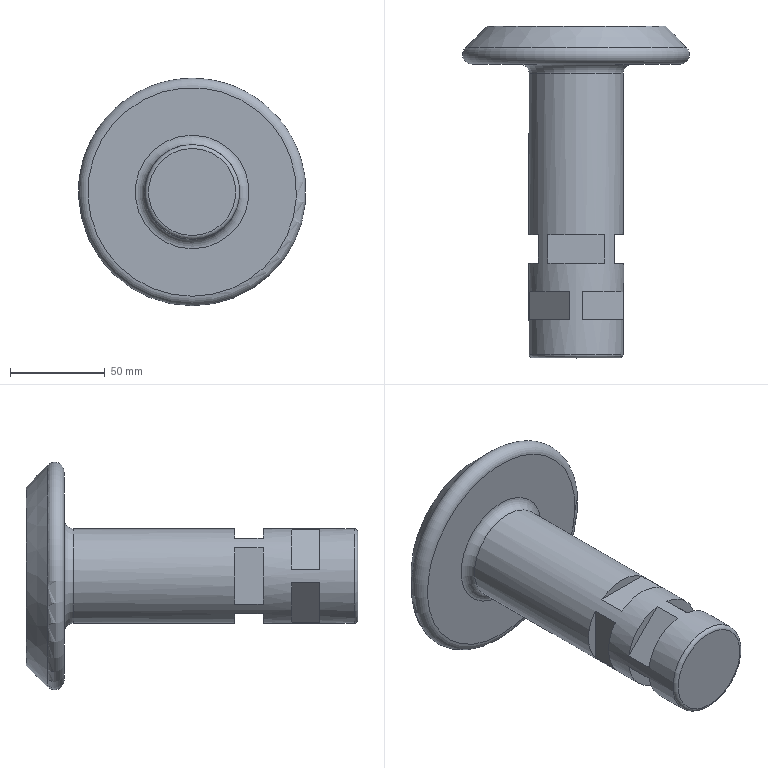Part | NX | features solid 2 | 1 solid | 32 faces | box 120 x 175 x 120 mm | volume 487590 mm3 | plane 27 | torus 3 | cylinder 1 | cone 1 | commonest cylinder face diameters 50 x1
STEP:
#1=CARTESIAN_POINT('',(745.,430.,-50.));
#2=VERTEX_POINT('',#1);
#3=CARTESIAN_POINT('',(745.,430.,-75.));
#4=DIRECTION('',(0.,-1.,0.));
#5=DIRECTION('',(0.,0.,1.));
#6=AXIS2_PLACEMENT_3D('',#3,#4,#5);
#7=CIRCLE('',#6,25.);
#8=EDGE_CURVE('',#2,#2,#7,.F.);
#9=ORIENTED_EDGE('',*,*,#8,.F.);
#10=EDGE_LOOP('',(#9));
#11=FACE_BOUND('',#10,.T.);
#12=CARTESIAN_POINT('',(741.464,300.,-50.251));
#13=VERTEX_POINT('',#12);
#14=CARTESIAN_POINT('',(741.464,315.,-50.251));
#15=VERTEX_POINT('',#14);
#16=CARTESIAN_POINT('',(741.464,435.,-50.251));
#17=DIRECTION('',(0.,-1.,0.));
#18=VECTOR('',#17,1000.);
#19=LINE('',#16,#18);
#20=EDGE_CURVE('',#13,#15,#19,.F.);
#21=ORIENTED_EDGE('',*,*,#20,.F.);
#22=CARTESIAN_POINT('',(720.251,300.,-71.464));
#23=VERTEX_POINT('',#22);
#24=CARTESIAN_POINT('',(745.,300.,-75.));
#25=DIRECTION('',(0.,-1.,0.));
#26=DIRECTION('',(0.,0.,1.));
#27=AXIS2_PLACEMENT_3D('',#24,#25,#26);
#28=CIRCLE('',#27,25.);
#29=EDGE_CURVE('',#23,#13,#28,.F.);
#30=ORIENTED_EDGE('',*,*,#29,.F.);
#31=CARTESIAN_POINT('',(720.251,315.,-71.464));
#32=VERTEX_POINT('',#31);
#33=CARTESIAN_POINT('',(720.251,435.,-71.464));
#34=DIRECTION('',(0.,-1.,0.));
#35=VECTOR('',#34,1000.);
#36=LINE('',#33,#35);
#37=EDGE_CURVE('',#32,#23,#36,.T.);
#38=ORIENTED_EDGE('',*,*,#37,.F.);
#39=CARTESIAN_POINT('',(745.,315.,-75.));
#40=DIRECTION('',(0.,-1.,0.));
#41=DIRECTION('',(0.,0.,1.));
#42=AXIS2_PLACEMENT_3D('',#39,#40,#41);
#43=CIRCLE('',#42,25.);
#44=EDGE_CURVE('',#15,#32,#43,.T.);
#45=ORIENTED_EDGE('',*,*,#44,.F.);
#46=EDGE_LOOP('',(#21,#30,#38,#45));
#47=FACE_BOUND('',#46,.T.);
#48=CARTESIAN_POINT('',(720.251,300.,-78.536));
#49=VERTEX_POINT('',#48);
#50=CARTESIAN_POINT('',(720.251,315.,-78.536));
#51=VERTEX_POINT('',#50);
#52=CARTESIAN_POINT('',(720.251,435.,-78.536));
#53=DIRECTION('',(0.,-1.,0.));
#54=VECTOR('',#53,1000.);
#55=LINE('',#52,#54);
#56=EDGE_CURVE('',#49,#51,#55,.F.);
#57=ORIENTED_EDGE('',*,*,#56,.F.);
#58=CARTESIAN_POINT('',(741.464,300.,-99.749));
#59=VERTEX_POINT('',#58);
#60=CARTESIAN_POINT('',(745.,300.,-75.));
#61=DIRECTION('',(0.,-1.,0.));
#62=DIRECTION('',(0.,0.,1.));
#63=AXIS2_PLACEMENT_3D('',#60,#61,#62);
#64=CIRCLE('',#63,25.);
#65=EDGE_CURVE('',#59,#49,#64,.F.);
#66=ORIENTED_EDGE('',*,*,#65,.F.);
#67=CARTESIAN_POINT('',(741.464,315.,-99.749));
#68=VERTEX_POINT('',#67);
#69=CARTESIAN_POINT('',(741.464,435.,-99.749));
#70=DIRECTION('',(0.,-1.,0.));
#71=VECTOR('',#70,1000.);
#72=LINE('',#69,#71);
#73=EDGE_CURVE('',#68,#59,#72,.T.);
#74=ORIENTED_EDGE('',*,*,#73,.F.);
#75=CARTESIAN_POINT('',(745.,315.,-75.));
#76=DIRECTION('',(0.,-1.,0.));
#77=DIRECTION('',(0.,0.,1.));
#78=AXIS2_PLACEMENT_3D('',#75,#76,#77);
#79=CIRCLE('',#78,25.);
#80=EDGE_CURVE('',#51,#68,#79,.T.);
#81=ORIENTED_EDGE('',*,*,#80,.F.);
#82=EDGE_LOOP('',(#57,#66,#74,#81));
#83=FACE_BOUND('',#82,.T.);
#84=CARTESIAN_POINT('',(725.,330.,-60.));
#85=VERTEX_POINT('',#84);
#86=CARTESIAN_POINT('',(725.,345.,-60.));
#87=VERTEX_POINT('',#86);
#88=CARTESIAN_POINT('',(725.,435.,-60.));
#89=DIRECTION('',(0.,-1.,0.));
#90=VECTOR('',#89,1000.);
#91=LINE('',#88,#90);
#92=EDGE_CURVE('',#85,#87,#91,.F.);
#93=ORIENTED_EDGE('',*,*,#92,.F.);
#94=CARTESIAN_POINT('',(725.,330.,-90.));
#95=VERTEX_POINT('',#94);
#96=CARTESIAN_POINT('',(745.,330.,-75.));
#97=DIRECTION('',(0.,-1.,0.));
#98=DIRECTION('',(0.,0.,1.));
#99=AXIS2_PLACEMENT_3D('',#96,#97,#98);
#100=CIRCLE('',#99,25.);
#101=EDGE_CURVE('',#95,#85,#100,.F.);
#102=ORIENTED_EDGE('',*,*,#101,.F.);
#103=CARTESIAN_POINT('',(725.,345.,-90.));
#104=VERTEX_POINT('',#103);
#105=CARTESIAN_POINT('',(725.,435.,-90.));
#106=DIRECTION('',(0.,-1.,0.));
#107=VECTOR('',#106,1000.);
#108=LINE('',#105,#107);
#109=EDGE_CURVE('',#104,#95,#108,.T.);
#110=ORIENTED_EDGE('',*,*,#109,.F.);
#111=CARTESIAN_POINT('',(745.,345.,-75.));
#112=DIRECTION('',(0.,-1.,0.));
#113=DIRECTION('',(0.,0.,1.));
#114=AXIS2_PLACEMENT_3D('',#111,#112,#113);
#115=CIRCLE('',#114,25.);
#116=EDGE_CURVE('',#87,#104,#115,.T.);
#117=ORIENTED_EDGE('',*,*,#116,.F.);
#118=EDGE_LOOP('',(#93,#102,#110,#117));
#119=FACE_BOUND('',#118,.T.);
#120=CARTESIAN_POINT('',(760.,345.,-55.));
#121=VERTEX_POINT('',#120);
#122=CARTESIAN_POINT('',(730.,345.,-55.));
#123=VERTEX_POINT('',#122);
#124=CARTESIAN_POINT('',(745.,345.,-75.));
#125=DIRECTION('',(0.,-1.,0.));
#126=DIRECTION('',(0.,0.,1.));
#127=AXIS2_PLACEMENT_3D('',#124,#125,#126);
#128=CIRCLE('',#127,25.);
#129=EDGE_CURVE('',#121,#123,#128,.T.);
#130=ORIENTED_EDGE('',*,*,#129,.F.);
#131=CARTESIAN_POINT('',(760.,330.,-55.));
#132=VERTEX_POINT('',#131);
#133=CARTESIAN_POINT('',(760.,435.,-55.));
#134=DIRECTION('',(0.,-1.,0.));
#135=VECTOR('',#134,1000.);
#136=LINE('',#133,#135);
#137=EDGE_CURVE('',#132,#121,#136,.F.);
#138=ORIENTED_EDGE('',*,*,#137,.F.);
#139=CARTESIAN_POINT('',(730.,330.,-55.));
#140=VERTEX_POINT('',#139);
#141=CARTESIAN_POINT('',(745.,330.,-75.));
#142=DIRECTION('',(0.,-1.,0.));
#143=DIRECTION('',(0.,0.,1.));
#144=AXIS2_PLACEMENT_3D('',#141,#142,#143);
#145=CIRCLE('',#144,25.);
#146=EDGE_CURVE('',#140,#132,#145,.F.);
#147=ORIENTED_EDGE('',*,*,#146,.F.);
#148=CARTESIAN_POINT('',(730.,435.,-55.));
#149=DIRECTION('',(0.,-1.,0.));
#150=VECTOR('',#149,1000.);
#151=LINE('',#148,#150);
#152=EDGE_CURVE('',#123,#140,#151,.T.);
#153=ORIENTED_EDGE('',*,*,#152,.F.);
#154=EDGE_LOOP('',(#130,#138,#147,#153));
#155=FACE_BOUND('',#154,.T.);
#156=CARTESIAN_POINT('',(745.,282.,-50.));
#157=VERTEX_POINT('',#156);
#158=CARTESIAN_POINT('',(745.,282.,-75.));
#159=DIRECTION('',(0.,-1.,0.));
#160=DIRECTION('',(0.,0.,1.));
#161=AXIS2_PLACEMENT_3D('',#158,#159,#160);
#162=CIRCLE('',#161,25.);
#163=EDGE_CURVE('',#157,#157,#162,.T.);
#164=ORIENTED_EDGE('',*,*,#163,.F.);
#165=EDGE_LOOP('',(#164));
#166=FACE_BOUND('',#165,.T.);
#167=CARTESIAN_POINT('',(760.,345.,-95.));
#168=VERTEX_POINT('',#167);
#169=CARTESIAN_POINT('',(730.,345.,-95.));
#170=VERTEX_POINT('',#169);
#171=CARTESIAN_POINT('',(745.,345.,-75.));
#172=DIRECTION('',(0.,-1.,0.));
#173=DIRECTION('',(0.,0.,1.));
#174=AXIS2_PLACEMENT_3D('',#171,#172,#173);
#175=CIRCLE('',#174,25.);
#176=EDGE_CURVE('',#168,#170,#175,.F.);
#177=ORIENTED_EDGE('',*,*,#176,.T.);
#178=CARTESIAN_POINT('',(730.,330.,-95.));
#179=VERTEX_POINT('',#178);
#180=CARTESIAN_POINT('',(730.,435.,-95.));
#181=DIRECTION('',(0.,-1.,0.));
#182=VECTOR('',#181,1000.);
#183=LINE('',#180,#182);
#184=EDGE_CURVE('',#170,#179,#183,.T.);
#185=ORIENTED_EDGE('',*,*,#184,.T.);
#186=CARTESIAN_POINT('',(760.,330.,-95.));
#187=VERTEX_POINT('',#186);
#188=CARTESIAN_POINT('',(745.,330.,-75.));
#189=DIRECTION('',(0.,-1.,0.));
#190=DIRECTION('',(0.,0.,1.));
#191=AXIS2_PLACEMENT_3D('',#188,#189,#190);
#192=CIRCLE('',#191,25.);
#193=EDGE_CURVE('',#179,#187,#192,.T.);
#194=ORIENTED_EDGE('',*,*,#193,.T.);
#195=CARTESIAN_POINT('',(760.,435.,-95.));
#196=DIRECTION('',(0.,-1.,0.));
#197=VECTOR('',#196,1000.);
#198=LINE('',#195,#197);
#199=EDGE_CURVE('',#187,#168,#198,.F.);
#200=ORIENTED_EDGE('',*,*,#199,.T.);
#201=EDGE_LOOP('',(#177,#185,#194,#200));
#202=FACE_BOUND('',#201,.T.);
#203=CARTESIAN_POINT('',(765.,345.,-60.));
#204=VERTEX_POINT('',#203);
#205=CARTESIAN_POINT('',(765.,345.,-90.));
#206=VERTEX_POINT('',#205);
#207=CARTESIAN_POINT('',(745.,345.,-75.));
#208=DIRECTION('',(0.,-1.,0.));
#209=DIRECTION('',(0.,0.,1.));
#210=AXIS2_PLACEMENT_3D('',#207,#208,#209);
#211=CIRCLE('',#210,25.);
#212=EDGE_CURVE('',#204,#206,#211,.F.);
#213=ORIENTED_EDGE('',*,*,#212,.T.);
#214=CARTESIAN_POINT('',(765.,330.,-90.));
#215=VERTEX_POINT('',#214);
#216=CARTESIAN_POINT('',(765.,435.,-90.));
#217=DIRECTION('',(0.,-1.,0.));
#218=VECTOR('',#217,1000.);
#219=LINE('',#216,#218);
#220=EDGE_CURVE('',#206,#215,#219,.T.);
#221=ORIENTED_EDGE('',*,*,#220,.T.);
#222=CARTESIAN_POINT('',(765.,330.,-60.));
#223=VERTEX_POINT('',#222);
#224=CARTESIAN_POINT('',(745.,330.,-75.));
#225=DIRECTION('',(0.,-1.,0.));
#226=DIRECTION('',(0.,0.,1.));
#227=AXIS2_PLACEMENT_3D('',#224,#225,#226);
#228=CIRCLE('',#227,25.);
#229=EDGE_CURVE('',#215,#223,#228,.T.);
#230=ORIENTED_EDGE('',*,*,#229,.T.);
#231=CARTESIAN_POINT('',(765.,435.,-60.));
#232=DIRECTION('',(0.,-1.,0.));
#233=VECTOR('',#232,1000.);
#234=LINE('',#231,#233);
#235=EDGE_CURVE('',#223,#204,#234,.F.);
#236=ORIENTED_EDGE('',*,*,#235,.T.);
#237=EDGE_LOOP('',(#213,#221,#230,#236));
#238=FACE_BOUND('',#237,.T.);
#239=CARTESIAN_POINT('',(748.536,315.,-50.251));
#240=VERTEX_POINT('',#239);
#241=CARTESIAN_POINT('',(769.749,315.,-71.464));
#242=VERTEX_POINT('',#241);
#243=CARTESIAN_POINT('',(745.,315.,-75.));
#244=DIRECTION('',(0.,-1.,0.));
#245=DIRECTION('',(0.,0.,1.));
#246=AXIS2_PLACEMENT_3D('',#243,#244,#245);
#247=CIRCLE('',#246,25.);
#248=EDGE_CURVE('',#240,#242,#247,.F.);
#249=ORIENTED_EDGE('',*,*,#248,.T.);
#250=CARTESIAN_POINT('',(769.749,300.,-71.464));
#251=VERTEX_POINT('',#250);
#252=CARTESIAN_POINT('',(769.749,435.,-71.464));
#253=DIRECTION('',(0.,-1.,0.));
#254=VECTOR('',#253,1000.);
#255=LINE('',#252,#254);
#256=EDGE_CURVE('',#242,#251,#255,.T.);
#257=ORIENTED_EDGE('',*,*,#256,.T.);
#258=CARTESIAN_POINT('',(748.536,300.,-50.251));
#259=VERTEX_POINT('',#258);
#260=CARTESIAN_POINT('',(745.,300.,-75.));
#261=DIRECTION('',(0.,-1.,0.));
#262=DIRECTION('',(0.,0.,1.));
#263=AXIS2_PLACEMENT_3D('',#260,#261,#262);
#264=CIRCLE('',#263,25.);
#265=EDGE_CURVE('',#251,#259,#264,.T.);
#266=ORIENTED_EDGE('',*,*,#265,.T.);
#267=CARTESIAN_POINT('',(748.536,435.,-50.251));
#268=DIRECTION('',(0.,-1.,0.));
#269=VECTOR('',#268,1000.);
#270=LINE('',#267,#269);
#271=EDGE_CURVE('',#259,#240,#270,.F.);
#272=ORIENTED_EDGE('',*,*,#271,.T.);
#273=EDGE_LOOP('',(#249,#257,#266,#272));
#274=FACE_BOUND('',#273,.T.);
#275=CARTESIAN_POINT('',(769.749,315.,-78.536));
#276=VERTEX_POINT('',#275);
#277=CARTESIAN_POINT('',(748.536,315.,-99.749));
#278=VERTEX_POINT('',#277);
#279=CARTESIAN_POINT('',(745.,315.,-75.));
#280=DIRECTION('',(0.,-1.,0.));
#281=DIRECTION('',(0.,0.,1.));
#282=AXIS2_PLACEMENT_3D('',#279,#280,#281);
#283=CIRCLE('',#282,25.);
#284=EDGE_CURVE('',#276,#278,#283,.F.);
#285=ORIENTED_EDGE('',*,*,#284,.T.);
#286=CARTESIAN_POINT('',(748.536,300.,-99.749));
#287=VERTEX_POINT('',#286);
#288=CARTESIAN_POINT('',(748.536,435.,-99.749));
#289=DIRECTION('',(0.,-1.,0.));
#290=VECTOR('',#289,1000.);
#291=LINE('',#288,#290);
#292=EDGE_CURVE('',#278,#287,#291,.T.);
#293=ORIENTED_EDGE('',*,*,#292,.T.);
#294=CARTESIAN_POINT('',(769.749,300.,-78.536));
#295=VERTEX_POINT('',#294);
#296=CARTESIAN_POINT('',(745.,300.,-75.));
#297=DIRECTION('',(0.,-1.,0.));
#298=DIRECTION('',(0.,0.,1.));
#299=AXIS2_PLACEMENT_3D('',#296,#297,#298);
#300=CIRCLE('',#299,25.);
#301=EDGE_CURVE('',#287,#295,#300,.T.);
#302=ORIENTED_EDGE('',*,*,#301,.T.);
#303=CARTESIAN_POINT('',(769.749,435.,-78.536));
#304=DIRECTION('',(0.,-1.,0.));
#305=VECTOR('',#304,1000.);
#306=LINE('',#303,#305);
#307=EDGE_CURVE('',#295,#276,#306,.F.);
#308=ORIENTED_EDGE('',*,*,#307,.T.);
#309=EDGE_LOOP('',(#285,#293,#302,#308));
#310=FACE_BOUND('',#309,.T.);
#311=CARTESIAN_POINT('',(745.,435.,-75.));
#312=DIRECTION('',(0.,-1.,0.));
#313=DIRECTION('',(0.,0.,-1.));
#314=AXIS2_PLACEMENT_3D('',#311,#312,#313);
#315=CYLINDRICAL_SURFACE('',#314,25.);
#316=ADVANCED_FACE('',(#11,#47,#83,#119,#155,#166,#202,#238,#274,#310),#315,.T.);
#317=CARTESIAN_POINT('',(745.,280.,-52.));
#318=VERTEX_POINT('',#317);
#319=CARTESIAN_POINT('',(745.,280.,-75.));
#320=DIRECTION('',(0.,-1.,0.));
#321=DIRECTION('',(0.,0.,1.));
#322=AXIS2_PLACEMENT_3D('',#319,#320,#321);
#323=CIRCLE('',#322,23.);
#324=EDGE_CURVE('',#318,#318,#323,.F.);
#325=ORIENTED_EDGE('',*,*,#324,.F.);
#326=EDGE_LOOP('',(#325));
#327=FACE_BOUND('',#326,.T.);
#328=CARTESIAN_POINT('',(720.,280.,-75.));
#329=DIRECTION('',(0.,1.,0.));
#330=DIRECTION('',(0.,0.,1.));
#331=AXIS2_PLACEMENT_3D('',#328,#329,#330);
#332=PLANE('',#331);
#333=ADVANCED_FACE('',(#327),#332,.F.);
#334=CARTESIAN_POINT('',(745.,435.,-45.));
#335=VERTEX_POINT('',#334);
#336=CARTESIAN_POINT('',(745.,435.,-75.));
#337=DIRECTION('',(0.,-1.,0.));
#338=DIRECTION('',(0.,0.,1.));
#339=AXIS2_PLACEMENT_3D('',#336,#337,#338);
#340=CIRCLE('',#339,30.);
#341=EDGE_CURVE('',#335,#335,#340,.T.);
#342=ORIENTED_EDGE('',*,*,#341,.F.);
#343=EDGE_LOOP('',(#342));
#344=FACE_BOUND('',#343,.T.);
#345=CARTESIAN_POINT('',(745.,435.,-130.));
#346=VERTEX_POINT('',#345);
#347=CARTESIAN_POINT('',(745.,435.,-75.));
#348=DIRECTION('',(0.,1.,0.));
#349=DIRECTION('',(0.,0.,-1.));
#350=AXIS2_PLACEMENT_3D('',#347,#348,#349);
#351=CIRCLE('',#350,55.);
#352=EDGE_CURVE('',#346,#346,#351,.T.);
#353=ORIENTED_EDGE('',*,*,#352,.F.);
#354=EDGE_LOOP('',(#353));
#355=FACE_BOUND('',#354,.T.);
#356=CARTESIAN_POINT('',(690.,435.,-75.));
#357=DIRECTION('',(0.,1.,0.));
#358=DIRECTION('',(0.,0.,1.));
#359=AXIS2_PLACEMENT_3D('',#356,#357,#358);
#360=PLANE('',#359);
#361=ADVANCED_FACE('',(#344,#355),#360,.F.);
#362=CARTESIAN_POINT('',(745.,443.536,-133.536));
#363=VERTEX_POINT('',#362);
#364=CARTESIAN_POINT('',(745.,443.536,-75.));
#365=DIRECTION('',(0.,1.,0.));
#366=DIRECTION('',(0.,0.,-1.));
#367=AXIS2_PLACEMENT_3D('',#364,#365,#366);
#368=CIRCLE('',#367,58.536);
#369=EDGE_CURVE('',#363,#363,#368,.T.);
#370=ORIENTED_EDGE('',*,*,#369,.T.);
#371=EDGE_LOOP('',(#370));
#372=FACE_BOUND('',#371,.T.);
#373=CARTESIAN_POINT('',(745.,455.,-122.071));
#374=VERTEX_POINT('',#373);
#375=CARTESIAN_POINT('',(745.,455.,-75.));
#376=DIRECTION('',(0.,1.,0.));
#377=DIRECTION('',(0.,0.,-1.));
#378=AXIS2_PLACEMENT_3D('',#375,#376,#377);
#379=CIRCLE('',#378,47.071);
#380=EDGE_CURVE('',#374,#374,#379,.T.);
#381=ORIENTED_EDGE('',*,*,#380,.F.);
#382=EDGE_LOOP('',(#381));
#383=FACE_BOUND('',#382,.T.);
#384=CARTESIAN_POINT('',(745.,455.,-75.));
#385=DIRECTION('',(0.,-1.,0.));
#386=DIRECTION('',(0.,0.,-1.));
#387=AXIS2_PLACEMENT_3D('',#384,#385,#386);
#388=CONICAL_SURFACE('',#387,47.071,0.7854);
#389=ADVANCED_FACE('',(#372,#383),#388,.T.);
#390=ORIENTED_EDGE('',*,*,#380,.T.);
#391=EDGE_LOOP('',(#390));
#392=FACE_BOUND('',#391,.T.);
#393=CARTESIAN_POINT('',(745.,455.,-75.));
#394=DIRECTION('',(0.,-1.,0.));
#395=DIRECTION('',(0.,0.,-1.));
#396=AXIS2_PLACEMENT_3D('',#393,#394,#395);
#397=PLANE('',#396);
#398=ADVANCED_FACE('',(#392),#397,.F.);
#399=ORIENTED_EDGE('',*,*,#369,.F.);
#400=EDGE_LOOP('',(#399));
#401=FACE_BOUND('',#400,.T.);
#402=ORIENTED_EDGE('',*,*,#352,.T.);
#403=EDGE_LOOP('',(#402));
#404=FACE_BOUND('',#403,.T.);
#405=CARTESIAN_POINT('',(745.,440.,-75.));
#406=DIRECTION('',(0.,-1.,0.));
#407=DIRECTION('',(0.,0.,-1.));
#408=AXIS2_PLACEMENT_3D('',#405,#406,#407);
#409=TOROIDAL_SURFACE('',#408,55.,5.);
#410=ADVANCED_FACE('',(#401,#404),#409,.T.);
#411=ORIENTED_EDGE('',*,*,#163,.T.);
#412=EDGE_LOOP('',(#411));
#413=FACE_BOUND('',#412,.T.);
#414=ORIENTED_EDGE('',*,*,#324,.T.);
#415=EDGE_LOOP('',(#414));
#416=FACE_BOUND('',#415,.T.);
#417=CARTESIAN_POINT('',(745.,282.,-75.));
#418=DIRECTION('',(0.,1.,0.));
#419=DIRECTION('',(0.,0.,1.));
#420=AXIS2_PLACEMENT_3D('',#417,#418,#419);
#421=TOROIDAL_SURFACE('',#420,23.,2.);
#422=ADVANCED_FACE('',(#413,#416),#421,.T.);
#423=CARTESIAN_POINT('',(765.,345.,-95.));
#424=DIRECTION('',(-1.,0.,0.));
#425=VECTOR('',#424,1000.);
#426=LINE('',#423,#425);
#427=EDGE_CURVE('',#168,#170,#426,.T.);
#428=ORIENTED_EDGE('',*,*,#427,.T.);
#429=ORIENTED_EDGE('',*,*,#176,.F.);
#430=EDGE_LOOP('',(#428,#429));
#431=FACE_BOUND('',#430,.T.);
#432=CARTESIAN_POINT('',(765.,345.,-75.));
#433=DIRECTION('',(0.,1.,0.));
#434=DIRECTION('',(-1.,0.,0.));
#435=AXIS2_PLACEMENT_3D('',#432,#433,#434);
#436=PLANE('',#435);
#437=ADVANCED_FACE('',(#431),#436,.F.);
#438=CARTESIAN_POINT('',(765.,330.,-95.));
#439=DIRECTION('',(-1.,0.,0.));
#440=VECTOR('',#439,1000.);
#441=LINE('',#438,#440);
#442=EDGE_CURVE('',#187,#179,#441,.T.);
#443=ORIENTED_EDGE('',*,*,#442,.F.);
#444=ORIENTED_EDGE('',*,*,#193,.F.);
#445=EDGE_LOOP('',(#443,#444));
#446=FACE_BOUND('',#445,.T.);
#447=CARTESIAN_POINT('',(765.,330.,-75.));
#448=DIRECTION('',(0.,1.,0.));
#449=DIRECTION('',(-1.,0.,0.));
#450=AXIS2_PLACEMENT_3D('',#447,#448,#449);
#451=PLANE('',#450);
#452=ADVANCED_FACE('',(#446),#451,.T.);
#453=ORIENTED_EDGE('',*,*,#184,.F.);
#454=ORIENTED_EDGE('',*,*,#427,.F.);
#455=ORIENTED_EDGE('',*,*,#199,.F.);
#456=ORIENTED_EDGE('',*,*,#442,.T.);
#457=EDGE_LOOP('',(#453,#454,#455,#456));
#458=FACE_BOUND('',#457,.T.);
#459=CARTESIAN_POINT('',(765.,345.,-95.));
#460=DIRECTION('',(0.,0.,-1.));
#461=DIRECTION('',(-1.,0.,0.));
#462=AXIS2_PLACEMENT_3D('',#459,#460,#461);
#463=PLANE('',#462);
#464=ADVANCED_FACE('',(#458),#463,.T.);
#465=ORIENTED_EDGE('',*,*,#129,.T.);
#466=CARTESIAN_POINT('',(765.,345.,-55.));
#467=DIRECTION('',(-1.,0.,0.));
#468=VECTOR('',#467,1000.);
#469=LINE('',#466,#468);
#470=EDGE_CURVE('',#121,#123,#469,.T.);
#471=ORIENTED_EDGE('',*,*,#470,.F.);
#472=EDGE_LOOP('',(#465,#471));
#473=FACE_BOUND('',#472,.T.);
#474=CARTESIAN_POINT('',(765.,345.,-75.));
#475=DIRECTION('',(0.,1.,0.));
#476=DIRECTION('',(-1.,0.,0.));
#477=AXIS2_PLACEMENT_3D('',#474,#475,#476);
#478=PLANE('',#477);
#479=ADVANCED_FACE('',(#473),#478,.F.);
#480=ORIENTED_EDGE('',*,*,#146,.T.);
#481=CARTESIAN_POINT('',(765.,330.,-55.));
#482=DIRECTION('',(-1.,0.,0.));
#483=VECTOR('',#482,1000.);
#484=LINE('',#481,#483);
#485=EDGE_CURVE('',#132,#140,#484,.T.);
#486=ORIENTED_EDGE('',*,*,#485,.T.);
#487=EDGE_LOOP('',(#480,#486));
#488=FACE_BOUND('',#487,.T.);
#489=CARTESIAN_POINT('',(765.,330.,-75.));
#490=DIRECTION('',(0.,1.,0.));
#491=DIRECTION('',(-1.,0.,0.));
#492=AXIS2_PLACEMENT_3D('',#489,#490,#491);
#493=PLANE('',#492);
#494=ADVANCED_FACE('',(#488),#493,.T.);
#495=ORIENTED_EDGE('',*,*,#470,.T.);
#496=ORIENTED_EDGE('',*,*,#152,.T.);
#497=ORIENTED_EDGE('',*,*,#485,.F.);
#498=ORIENTED_EDGE('',*,*,#137,.T.);
#499=EDGE_LOOP('',(#495,#496,#497,#498));
#500=FACE_BOUND('',#499,.T.);
#501=CARTESIAN_POINT('',(765.,345.,-55.));
#502=DIRECTION('',(0.,0.,-1.));
#503=DIRECTION('',(-1.,0.,0.));
#504=AXIS2_PLACEMENT_3D('',#501,#502,#503);
#505=PLANE('',#504);
#506=ADVANCED_FACE('',(#500),#505,.F.);
#507=CARTESIAN_POINT('',(765.,345.,-55.));
#508=DIRECTION('',(0.,0.,-1.));
#509=VECTOR('',#508,1000.);
#510=LINE('',#507,#509);
#511=EDGE_CURVE('',#204,#206,#510,.T.);
#512=ORIENTED_EDGE('',*,*,#511,.T.);
#513=ORIENTED_EDGE('',*,*,#212,.F.);
#514=EDGE_LOOP('',(#512,#513));
#515=FACE_BOUND('',#514,.T.);
#516=CARTESIAN_POINT('',(745.,345.,-55.));
#517=DIRECTION('',(0.,1.,0.));
#518=DIRECTION('',(0.,0.,-1.));
#519=AXIS2_PLACEMENT_3D('',#516,#517,#518);
#520=PLANE('',#519);
#521=ADVANCED_FACE('',(#515),#520,.F.);
#522=CARTESIAN_POINT('',(765.,330.,-55.));
#523=DIRECTION('',(0.,0.,-1.));
#524=VECTOR('',#523,1000.);
#525=LINE('',#522,#524);
#526=EDGE_CURVE('',#223,#215,#525,.T.);
#527=ORIENTED_EDGE('',*,*,#526,.F.);
#528=ORIENTED_EDGE('',*,*,#229,.F.);
#529=EDGE_LOOP('',(#527,#528));
#530=FACE_BOUND('',#529,.T.);
#531=CARTESIAN_POINT('',(745.,330.,-55.));
#532=DIRECTION('',(0.,1.,0.));
#533=DIRECTION('',(0.,0.,-1.));
#534=AXIS2_PLACEMENT_3D('',#531,#532,#533);
#535=PLANE('',#534);
#536=ADVANCED_FACE('',(#530),#535,.T.);
#537=ORIENTED_EDGE('',*,*,#220,.F.);
#538=ORIENTED_EDGE('',*,*,#511,.F.);
#539=ORIENTED_EDGE('',*,*,#235,.F.);
#540=ORIENTED_EDGE('',*,*,#526,.T.);
#541=EDGE_LOOP('',(#537,#538,#539,#540));
#542=FACE_BOUND('',#541,.T.);
#543=CARTESIAN_POINT('',(765.,345.,-55.));
#544=DIRECTION('',(1.,0.,0.));
#545=DIRECTION('',(0.,0.,-1.));
#546=AXIS2_PLACEMENT_3D('',#543,#544,#545);
#547=PLANE('',#546);
#548=ADVANCED_FACE('',(#542),#547,.T.);
#549=CARTESIAN_POINT('',(725.,345.,-55.));
#550=DIRECTION('',(0.,0.,-1.));
#551=VECTOR('',#550,1000.);
#552=LINE('',#549,#551);
#553=EDGE_CURVE('',#87,#104,#552,.T.);
#554=ORIENTED_EDGE('',*,*,#553,.F.);
#555=ORIENTED_EDGE('',*,*,#116,.T.);
#556=EDGE_LOOP('',(#554,#555));
#557=FACE_BOUND('',#556,.T.);
#558=CARTESIAN_POINT('',(745.,345.,-55.));
#559=DIRECTION('',(0.,1.,0.));
#560=DIRECTION('',(0.,0.,-1.));
#561=AXIS2_PLACEMENT_3D('',#558,#559,#560);
#562=PLANE('',#561);
#563=ADVANCED_FACE('',(#557),#562,.F.);
#564=CARTESIAN_POINT('',(725.,330.,-55.));
#565=DIRECTION('',(0.,0.,-1.));
#566=VECTOR('',#565,1000.);
#567=LINE('',#564,#566);
#568=EDGE_CURVE('',#85,#95,#567,.T.);
#569=ORIENTED_EDGE('',*,*,#568,.T.);
#570=ORIENTED_EDGE('',*,*,#101,.T.);
#571=EDGE_LOOP('',(#569,#570));
#572=FACE_BOUND('',#571,.T.);
#573=CARTESIAN_POINT('',(745.,330.,-55.));
#574=DIRECTION('',(0.,1.,0.));
#575=DIRECTION('',(0.,0.,-1.));
#576=AXIS2_PLACEMENT_3D('',#573,#574,#575);
#577=PLANE('',#576);
#578=ADVANCED_FACE('',(#572),#577,.T.);
#579=ORIENTED_EDGE('',*,*,#553,.T.);
#580=ORIENTED_EDGE('',*,*,#109,.T.);
#581=ORIENTED_EDGE('',*,*,#568,.F.);
#582=ORIENTED_EDGE('',*,*,#92,.T.);
#583=EDGE_LOOP('',(#579,#580,#581,#582));
#584=FACE_BOUND('',#583,.T.);
#585=CARTESIAN_POINT('',(725.,345.,-55.));
#586=DIRECTION('',(1.,0.,0.));
#587=DIRECTION('',(0.,0.,-1.));
#588=AXIS2_PLACEMENT_3D('',#585,#586,#587);
#589=PLANE('',#588);
#590=ADVANCED_FACE('',(#584),#589,.F.);
#591=CARTESIAN_POINT('',(716.716,315.,-75.));
#592=DIRECTION('',(0.7071,0.,-0.7071));
#593=VECTOR('',#592,1000.);
#594=LINE('',#591,#593);
#595=EDGE_CURVE('',#51,#68,#594,.T.);
#596=ORIENTED_EDGE('',*,*,#595,.F.);
#597=ORIENTED_EDGE('',*,*,#80,.T.);
#598=EDGE_LOOP('',(#596,#597));
#599=FACE_BOUND('',#598,.T.);
#600=CARTESIAN_POINT('',(730.858,315.,-60.858));
#601=DIRECTION('',(0.,1.,0.));
#602=DIRECTION('',(0.7071,0.,-0.7071));
#603=AXIS2_PLACEMENT_3D('',#600,#601,#602);
#604=PLANE('',#603);
#605=ADVANCED_FACE('',(#599),#604,.F.);
#606=CARTESIAN_POINT('',(716.716,300.,-75.));
#607=DIRECTION('',(0.7071,0.,-0.7071));
#608=VECTOR('',#607,1000.);
#609=LINE('',#606,#608);
#610=EDGE_CURVE('',#49,#59,#609,.T.);
#611=ORIENTED_EDGE('',*,*,#610,.T.);
#612=ORIENTED_EDGE('',*,*,#65,.T.);
#613=EDGE_LOOP('',(#611,#612));
#614=FACE_BOUND('',#613,.T.);
#615=CARTESIAN_POINT('',(730.858,300.,-60.858));
#616=DIRECTION('',(0.,1.,0.));
#617=DIRECTION('',(0.7071,0.,-0.7071));
#618=AXIS2_PLACEMENT_3D('',#615,#616,#617);
#619=PLANE('',#618);
#620=ADVANCED_FACE('',(#614),#619,.T.);
#621=ORIENTED_EDGE('',*,*,#595,.T.);
#622=ORIENTED_EDGE('',*,*,#73,.T.);
#623=ORIENTED_EDGE('',*,*,#610,.F.);
#624=ORIENTED_EDGE('',*,*,#56,.T.);
#625=EDGE_LOOP('',(#621,#622,#623,#624));
#626=FACE_BOUND('',#625,.T.);
#627=CARTESIAN_POINT('',(716.716,315.,-75.));
#628=DIRECTION('',(0.7071,0.,0.7071));
#629=DIRECTION('',(0.7071,0.,-0.7071));
#630=AXIS2_PLACEMENT_3D('',#627,#628,#629);
#631=PLANE('',#630);
#632=ADVANCED_FACE('',(#626),#631,.F.);
#633=CARTESIAN_POINT('',(745.,315.,-46.716));
#634=DIRECTION('',(0.7071,0.,-0.7071));
#635=VECTOR('',#634,1000.);
#636=LINE('',#633,#635);
#637=EDGE_CURVE('',#240,#242,#636,.T.);
#638=ORIENTED_EDGE('',*,*,#637,.T.);
#639=ORIENTED_EDGE('',*,*,#248,.F.);
#640=EDGE_LOOP('',(#638,#639));
#641=FACE_BOUND('',#640,.T.);
#642=CARTESIAN_POINT('',(730.858,315.,-60.858));
#643=DIRECTION('',(0.,1.,0.));
#644=DIRECTION('',(0.7071,0.,-0.7071));
#645=AXIS2_PLACEMENT_3D('',#642,#643,#644);
#646=PLANE('',#645);
#647=ADVANCED_FACE('',(#641),#646,.F.);
#648=CARTESIAN_POINT('',(745.,300.,-46.716));
#649=DIRECTION('',(0.7071,0.,-0.7071));
#650=VECTOR('',#649,1000.);
#651=LINE('',#648,#650);
#652=EDGE_CURVE('',#259,#251,#651,.T.);
#653=ORIENTED_EDGE('',*,*,#652,.F.);
#654=ORIENTED_EDGE('',*,*,#265,.F.);
#655=EDGE_LOOP('',(#653,#654));
#656=FACE_BOUND('',#655,.T.);
#657=CARTESIAN_POINT('',(730.858,300.,-60.858));
#658=DIRECTION('',(0.,1.,0.));
#659=DIRECTION('',(0.7071,0.,-0.7071));
#660=AXIS2_PLACEMENT_3D('',#657,#658,#659);
#661=PLANE('',#660);
#662=ADVANCED_FACE('',(#656),#661,.T.);
#663=ORIENTED_EDGE('',*,*,#256,.F.);
#664=ORIENTED_EDGE('',*,*,#637,.F.);
#665=ORIENTED_EDGE('',*,*,#271,.F.);
#666=ORIENTED_EDGE('',*,*,#652,.T.);
#667=EDGE_LOOP('',(#663,#664,#665,#666));
#668=FACE_BOUND('',#667,.T.);
#669=CARTESIAN_POINT('',(745.,315.,-46.716));
#670=DIRECTION('',(0.7071,0.,0.7071));
#671=DIRECTION('',(0.7071,0.,-0.7071));
#672=AXIS2_PLACEMENT_3D('',#669,#670,#671);
#673=PLANE('',#672);
#674=ADVANCED_FACE('',(#668),#673,.T.);
#675=CARTESIAN_POINT('',(773.284,315.,-75.));
#676=DIRECTION('',(-0.7071,0.,-0.7071));
#677=VECTOR('',#676,1000.);
#678=LINE('',#675,#677);
#679=EDGE_CURVE('',#276,#278,#678,.T.);
#680=ORIENTED_EDGE('',*,*,#679,.T.);
#681=ORIENTED_EDGE('',*,*,#284,.F.);
#682=EDGE_LOOP('',(#680,#681));
#683=FACE_BOUND('',#682,.T.);
#684=CARTESIAN_POINT('',(759.142,315.,-60.858));
#685=DIRECTION('',(0.,1.,0.));
#686=DIRECTION('',(-0.7071,0.,-0.7071));
#687=AXIS2_PLACEMENT_3D('',#684,#685,#686);
#688=PLANE('',#687);
#689=ADVANCED_FACE('',(#683),#688,.F.);
#690=CARTESIAN_POINT('',(773.284,300.,-75.));
#691=DIRECTION('',(-0.7071,0.,-0.7071));
#692=VECTOR('',#691,1000.);
#693=LINE('',#690,#692);
#694=EDGE_CURVE('',#295,#287,#693,.T.);
#695=ORIENTED_EDGE('',*,*,#694,.F.);
#696=ORIENTED_EDGE('',*,*,#301,.F.);
#697=EDGE_LOOP('',(#695,#696));
#698=FACE_BOUND('',#697,.T.);
#699=CARTESIAN_POINT('',(759.142,300.,-60.858));
#700=DIRECTION('',(0.,1.,0.));
#701=DIRECTION('',(-0.7071,0.,-0.7071));
#702=AXIS2_PLACEMENT_3D('',#699,#700,#701);
#703=PLANE('',#702);
#704=ADVANCED_FACE('',(#698),#703,.T.);
#705=ORIENTED_EDGE('',*,*,#292,.F.);
#706=ORIENTED_EDGE('',*,*,#679,.F.);
#707=ORIENTED_EDGE('',*,*,#307,.F.);
#708=ORIENTED_EDGE('',*,*,#694,.T.);
#709=EDGE_LOOP('',(#705,#706,#707,#708));
#710=FACE_BOUND('',#709,.T.);
#711=CARTESIAN_POINT('',(773.284,315.,-75.));
#712=DIRECTION('',(0.7071,0.,-0.7071));
#713=DIRECTION('',(-0.7071,0.,-0.7071));
#714=AXIS2_PLACEMENT_3D('',#711,#712,#713);
#715=PLANE('',#714);
#716=ADVANCED_FACE('',(#710),#715,.T.);
#717=CARTESIAN_POINT('',(745.,315.,-46.716));
#718=DIRECTION('',(-0.7071,0.,-0.7071));
#719=VECTOR('',#718,1000.);
#720=LINE('',#717,#719);
#721=EDGE_CURVE('',#15,#32,#720,.T.);
#722=ORIENTED_EDGE('',*,*,#721,.F.);
#723=ORIENTED_EDGE('',*,*,#44,.T.);
#724=EDGE_LOOP('',(#722,#723));
#725=FACE_BOUND('',#724,.T.);
#726=CARTESIAN_POINT('',(759.142,315.,-60.858));
#727=DIRECTION('',(0.,1.,0.));
#728=DIRECTION('',(-0.7071,0.,-0.7071));
#729=AXIS2_PLACEMENT_3D('',#726,#727,#728);
#730=PLANE('',#729);
#731=ADVANCED_FACE('',(#725),#730,.F.);
#732=CARTESIAN_POINT('',(745.,300.,-46.716));
#733=DIRECTION('',(-0.7071,0.,-0.7071));
#734=VECTOR('',#733,1000.);
#735=LINE('',#732,#734);
#736=EDGE_CURVE('',#13,#23,#735,.T.);
#737=ORIENTED_EDGE('',*,*,#736,.T.);
#738=ORIENTED_EDGE('',*,*,#29,.T.);
#739=EDGE_LOOP('',(#737,#738));
#740=FACE_BOUND('',#739,.T.);
#741=CARTESIAN_POINT('',(759.142,300.,-60.858));
#742=DIRECTION('',(0.,1.,0.));
#743=DIRECTION('',(-0.7071,0.,-0.7071));
#744=AXIS2_PLACEMENT_3D('',#741,#742,#743);
#745=PLANE('',#744);
#746=ADVANCED_FACE('',(#740),#745,.T.);
#747=ORIENTED_EDGE('',*,*,#721,.T.);
#748=ORIENTED_EDGE('',*,*,#37,.T.);
#749=ORIENTED_EDGE('',*,*,#736,.F.);
#750=ORIENTED_EDGE('',*,*,#20,.T.);
#751=EDGE_LOOP('',(#747,#748,#749,#750));
#752=FACE_BOUND('',#751,.T.);
#753=CARTESIAN_POINT('',(745.,315.,-46.716));
#754=DIRECTION('',(0.7071,0.,-0.7071));
#755=DIRECTION('',(-0.7071,0.,-0.7071));
#756=AXIS2_PLACEMENT_3D('',#753,#754,#755);
#757=PLANE('',#756);
#758=ADVANCED_FACE('',(#752),#757,.F.);
#759=ORIENTED_EDGE('',*,*,#341,.T.);
#760=EDGE_LOOP('',(#759));
#761=FACE_BOUND('',#760,.T.);
#762=ORIENTED_EDGE('',*,*,#8,.T.);
#763=EDGE_LOOP('',(#762));
#764=FACE_BOUND('',#763,.T.);
#765=CARTESIAN_POINT('',(745.,430.,-75.));
#766=DIRECTION('',(0.,1.,0.));
#767=DIRECTION('',(0.,0.,1.));
#768=AXIS2_PLACEMENT_3D('',#765,#766,#767);
#769=TOROIDAL_SURFACE('',#768,30.,5.);
#770=ADVANCED_FACE('',(#761,#764),#769,.F.);
#771=CLOSED_SHELL('',(#316,#333,#361,#389,#398,#410,#422,#437,#452,#464,#479,#494,#506,#521,#536,#548,#563,#578,#590,#605,#620,#632,#647,#662,#674,#689,#704,#716,#731,#746,#758,#770));
#772=MANIFOLD_SOLID_BREP('',#771);
#773=(LENGTH_UNIT()NAMED_UNIT(*)SI_UNIT(.MILLI.,.METRE.));
#774=UNCERTAINTY_MEASURE_WITH_UNIT(LENGTH_MEASURE(0.00001),#773,'','');
#775=(NAMED_UNIT(*)PLANE_ANGLE_UNIT()SI_UNIT($,.RADIAN.));
#776=(NAMED_UNIT(*)SI_UNIT($,.STERADIAN.)SOLID_ANGLE_UNIT());
#777=(GEOMETRIC_REPRESENTATION_CONTEXT(3)GLOBAL_UNCERTAINTY_ASSIGNED_CONTEXT((#774))GLOBAL_UNIT_ASSIGNED_CONTEXT((#773,#775,#776))REPRESENTATION_CONTEXT('',''));
#778=ADVANCED_BREP_SHAPE_REPRESENTATION('',(#772),#777);